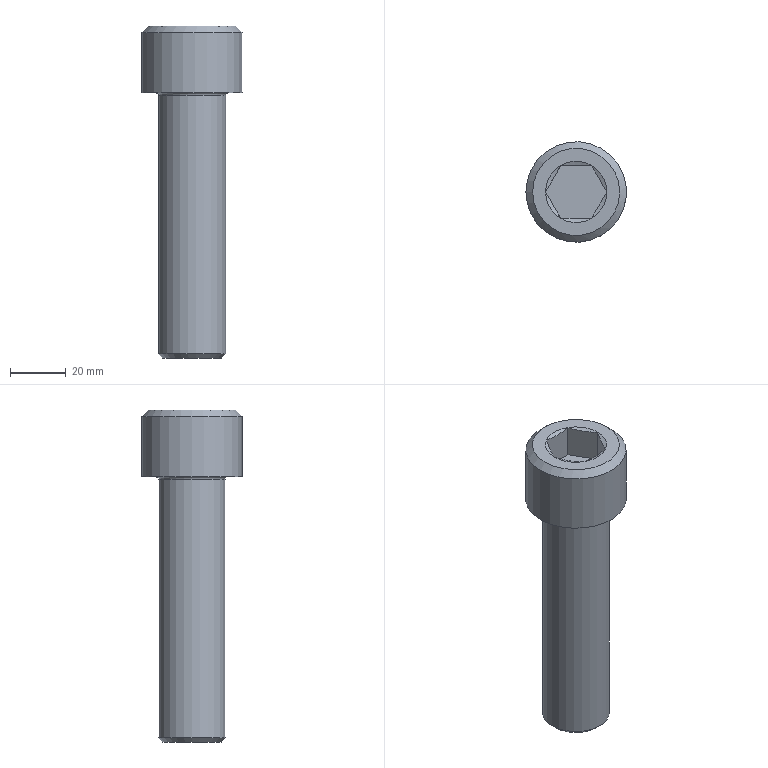Part | STEP file | solid 18 | 1 solid | 21 faces | box 36 x 36 x 119 mm | volume 63256 mm3 | plane 10 | sphere 6 | cylinder 2 | cone 2 | torus 1 | commonest cylinder face diameters 24 x1 36 x1